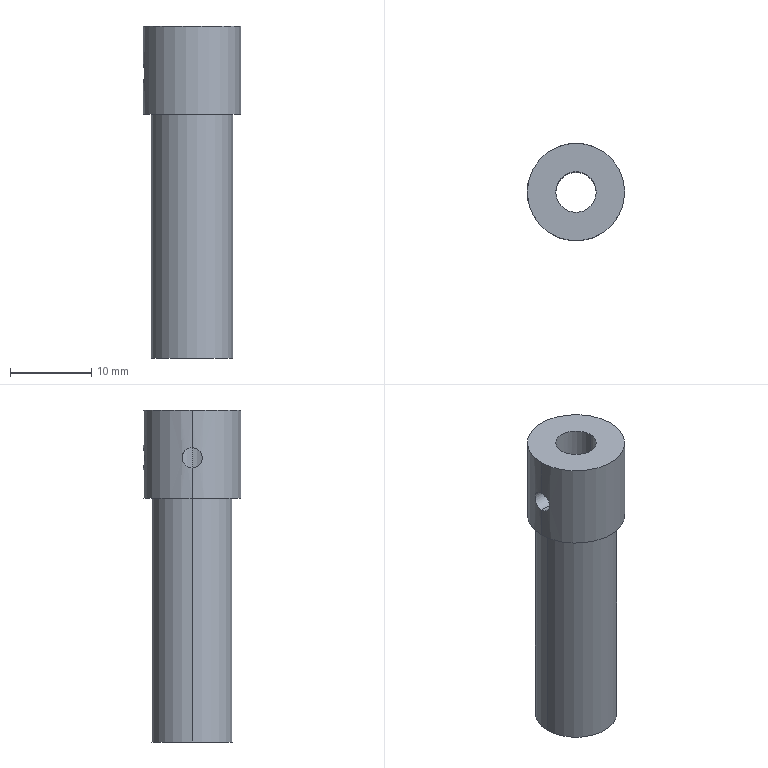Part | STEP file | 04-09 rotary shaft | 1 solid | 13 faces | box 12 x 12 x 40.9 mm | volume 2751 mm3 | cylinder 10 | plane 3 | commonest cylinder face diameters 2.5 x4 5 x2 10 x2 12 x2
STEP:
#1=CARTESIAN_POINT('',(-6.,0.,6.25));
#2=VERTEX_POINT('',#1);
#3=CARTESIAN_POINT('',(-6.,0.,3.75));
#4=VERTEX_POINT('',#3);
#5=CARTESIAN_POINT('',(-6.,0.,6.25));
#6=CARTESIAN_POINT('',(-6.,-0.1657,6.25));
#7=CARTESIAN_POINT('',(-5.993,-0.3282,6.217));
#8=CARTESIAN_POINT('',(-5.969,-0.6308,6.092));
#9=CARTESIAN_POINT('',(-5.952,-0.7692,5.999));
#10=CARTESIAN_POINT('',(-5.917,-0.9991,5.769));
#11=CARTESIAN_POINT('',(-5.9,-1.092,5.63));
#12=CARTESIAN_POINT('',(-5.876,-1.217,5.329));
#13=CARTESIAN_POINT('',(-5.868,-1.25,5.164));
#14=CARTESIAN_POINT('',(-5.868,-1.25,4.919));
#15=CARTESIAN_POINT('',(-5.87,-1.242,4.836));
#16=CARTESIAN_POINT('',(-5.877,-1.21,4.675));
#17=CARTESIAN_POINT('',(-5.882,-1.186,4.597));
#18=CARTESIAN_POINT('',(-5.9,-1.092,4.37));
#19=CARTESIAN_POINT('',(-5.917,-0.9999,4.232));
#20=CARTESIAN_POINT('',(-5.952,-0.7677,4.));
#21=CARTESIAN_POINT('',(-5.969,-0.63,3.908));
#22=CARTESIAN_POINT('',(-5.993,-0.3278,3.783));
#23=CARTESIAN_POINT('',(-6.,-0.1634,3.75));
#24=CARTESIAN_POINT('',(-6.,0.,3.75));
#25=B_SPLINE_CURVE_WITH_KNOTS('',3,(#5,#6,#7,#8,#9,#10,#11,#12,#13,#14,#15,#16,#17,#18,#19,#20,#21,#22,#23,#24),.UNSPECIFIED.,.F.,.F.,(4,2,2,2,2,2,2,2,2,4),(0.,0.0004899,0.0009797,0.00147,0.001959,0.002204,0.002449,0.002939,0.003429,0.003919),.UNSPECIFIED.);
#26=EDGE_CURVE('',#2,#4,#25,.T.);
#27=ORIENTED_EDGE('',*,*,#26,.F.);
#28=CARTESIAN_POINT('',(-2.5,0.,6.25));
#29=VERTEX_POINT('',#28);
#30=CARTESIAN_POINT('',(0.,0.,6.25));
#31=DIRECTION('',(1.,0.,0.));
#32=VECTOR('',#31,1000.);
#33=LINE('',#30,#32);
#34=EDGE_CURVE('',#2,#29,#33,.T.);
#35=ORIENTED_EDGE('',*,*,#34,.T.);
#36=CARTESIAN_POINT('',(-2.5,0.,3.75));
#37=VERTEX_POINT('',#36);
#38=CARTESIAN_POINT('',(-2.5,0.,3.75));
#39=CARTESIAN_POINT('',(-2.5,-0.08412,3.75));
#40=CARTESIAN_POINT('',(-2.496,-0.1666,3.758));
#41=CARTESIAN_POINT('',(-2.48,-0.3284,3.791));
#42=CARTESIAN_POINT('',(-2.468,-0.4085,3.816));
#43=CARTESIAN_POINT('',(-2.423,-0.635,3.911));
#44=CARTESIAN_POINT('',(-2.381,-0.7717,4.004));
#45=CARTESIAN_POINT('',(-2.295,-0.9981,4.231));
#46=CARTESIAN_POINT('',(-2.251,-1.09,4.367));
#47=CARTESIAN_POINT('',(-2.202,-1.184,4.592));
#48=CARTESIAN_POINT('',(-2.188,-1.209,4.672));
#49=CARTESIAN_POINT('',(-2.17,-1.242,4.834));
#50=CARTESIAN_POINT('',(-2.165,-1.25,4.916));
#51=CARTESIAN_POINT('',(-2.165,-1.25,5.165));
#52=CARTESIAN_POINT('',(-2.185,-1.216,5.332));
#53=CARTESIAN_POINT('',(-2.251,-1.089,5.634));
#54=CARTESIAN_POINT('',(-2.296,-0.9974,5.77));
#55=CARTESIAN_POINT('',(-2.381,-0.7706,5.997));
#56=CARTESIAN_POINT('',(-2.423,-0.6332,6.09));
#57=CARTESIAN_POINT('',(-2.482,-0.3331,6.216));
#58=CARTESIAN_POINT('',(-2.5,-0.166,6.25));
#59=CARTESIAN_POINT('',(-2.5,0.,6.25));
#60=B_SPLINE_CURVE_WITH_KNOTS('',3,(#38,#39,#40,#41,#42,#43,#44,#45,#46,#47,#48,#49,#50,#51,#52,#53,#54,#55,#56,#57,#58,#59),.UNSPECIFIED.,.F.,.F.,(4,2,2,2,2,2,2,2,2,2,4),(0.,0.0002485,0.000497,0.0009941,0.001491,0.00174,0.001988,0.002485,0.002982,0.003479,0.003976),.UNSPECIFIED.);
#61=EDGE_CURVE('',#37,#29,#60,.T.);
#62=ORIENTED_EDGE('',*,*,#61,.F.);
#63=CARTESIAN_POINT('',(0.,0.,3.75));
#64=DIRECTION('',(1.,0.,0.));
#65=VECTOR('',#64,1000.);
#66=LINE('',#63,#65);
#67=EDGE_CURVE('',#4,#37,#66,.T.);
#68=ORIENTED_EDGE('',*,*,#67,.F.);
#69=EDGE_LOOP('',(#27,#35,#62,#68));
#70=FACE_OUTER_BOUND('',#69,.T.);
#71=CARTESIAN_POINT('',(0.,0.,5.));
#72=DIRECTION('',(1.,0.,0.));
#73=DIRECTION('',(0.,0.,-1.));
#74=AXIS2_PLACEMENT_3D('',#71,#72,#73);
#75=CYLINDRICAL_SURFACE('',#74,1.25);
#76=ADVANCED_FACE('',(#70),#75,.F.);
#77=CARTESIAN_POINT('',(0.,6.,6.25));
#78=VERTEX_POINT('',#77);
#79=CARTESIAN_POINT('',(0.,6.,3.75));
#80=VERTEX_POINT('',#79);
#81=CARTESIAN_POINT('',(0.,6.,6.25));
#82=CARTESIAN_POINT('',(-0.1634,6.,6.25));
#83=CARTESIAN_POINT('',(-0.3283,5.993,6.217));
#84=CARTESIAN_POINT('',(-0.6292,5.969,6.092));
#85=CARTESIAN_POINT('',(-0.7681,5.952,6.));
#86=CARTESIAN_POINT('',(-0.9987,5.917,5.769));
#87=CARTESIAN_POINT('',(-1.091,5.9,5.632));
#88=CARTESIAN_POINT('',(-1.217,5.876,5.328));
#89=CARTESIAN_POINT('',(-1.25,5.868,5.166));
#90=CARTESIAN_POINT('',(-1.25,5.868,4.836));
#91=CARTESIAN_POINT('',(-1.217,5.876,4.672));
#92=CARTESIAN_POINT('',(-1.092,5.9,4.37));
#93=CARTESIAN_POINT('',(-0.9992,5.917,4.232));
#94=CARTESIAN_POINT('',(-0.7697,5.952,4.002));
#95=CARTESIAN_POINT('',(-0.6307,5.969,3.909));
#96=CARTESIAN_POINT('',(-0.33,5.993,3.783));
#97=CARTESIAN_POINT('',(-0.1656,6.,3.75));
#98=CARTESIAN_POINT('',(0.,6.,3.75));
#99=B_SPLINE_CURVE_WITH_KNOTS('',3,(#81,#82,#83,#84,#85,#86,#87,#88,#89,#90,#91,#92,#93,#94,#95,#96,#97,#98),.UNSPECIFIED.,.F.,.F.,(4,2,2,2,2,2,2,2,4),(0.003919,0.004409,0.004898,0.005388,0.005878,0.006367,0.006857,0.007347,0.007837),.UNSPECIFIED.);
#100=EDGE_CURVE('',#78,#80,#99,.T.);
#101=ORIENTED_EDGE('',*,*,#100,.F.);
#102=CARTESIAN_POINT('',(0.,2.5,6.25));
#103=VERTEX_POINT('',#102);
#104=CARTESIAN_POINT('',(0.,0.,6.25));
#105=DIRECTION('',(0.,-1.,0.));
#106=VECTOR('',#105,1000.);
#107=LINE('',#104,#106);
#108=EDGE_CURVE('',#78,#103,#107,.T.);
#109=ORIENTED_EDGE('',*,*,#108,.T.);
#110=CARTESIAN_POINT('',(0.,2.5,3.75));
#111=VERTEX_POINT('',#110);
#112=CARTESIAN_POINT('',(0.,2.5,3.75));
#113=CARTESIAN_POINT('',(-0.08412,2.5,3.75));
#114=CARTESIAN_POINT('',(-0.1666,2.496,3.758));
#115=CARTESIAN_POINT('',(-0.3284,2.48,3.791));
#116=CARTESIAN_POINT('',(-0.4085,2.468,3.816));
#117=CARTESIAN_POINT('',(-0.635,2.423,3.911));
#118=CARTESIAN_POINT('',(-0.7717,2.381,4.004));
#119=CARTESIAN_POINT('',(-0.9981,2.295,4.231));
#120=CARTESIAN_POINT('',(-1.09,2.251,4.367));
#121=CARTESIAN_POINT('',(-1.184,2.202,4.592));
#122=CARTESIAN_POINT('',(-1.209,2.188,4.672));
#123=CARTESIAN_POINT('',(-1.242,2.17,4.834));
#124=CARTESIAN_POINT('',(-1.25,2.165,4.916));
#125=CARTESIAN_POINT('',(-1.25,2.165,5.165));
#126=CARTESIAN_POINT('',(-1.216,2.185,5.332));
#127=CARTESIAN_POINT('',(-1.089,2.251,5.634));
#128=CARTESIAN_POINT('',(-0.9974,2.296,5.77));
#129=CARTESIAN_POINT('',(-0.7706,2.381,5.997));
#130=CARTESIAN_POINT('',(-0.6332,2.423,6.09));
#131=CARTESIAN_POINT('',(-0.3331,2.482,6.216));
#132=CARTESIAN_POINT('',(-0.166,2.5,6.25));
#133=CARTESIAN_POINT('',(0.,2.5,6.25));
#134=B_SPLINE_CURVE_WITH_KNOTS('',3,(#112,#113,#114,#115,#116,#117,#118,#119,#120,#121,#122,#123,#124,#125,#126,#127,#128,#129,#130,#131,#132,#133),.UNSPECIFIED.,.F.,.F.,(4,2,2,2,2,2,2,2,2,2,4),(0.,0.0002485,0.000497,0.0009941,0.001491,0.00174,0.001988,0.002485,0.002982,0.003479,0.003976),.UNSPECIFIED.);
#135=EDGE_CURVE('',#111,#103,#134,.T.);
#136=ORIENTED_EDGE('',*,*,#135,.F.);
#137=CARTESIAN_POINT('',(0.,0.,3.75));
#138=DIRECTION('',(0.,-1.,0.));
#139=VECTOR('',#138,1000.);
#140=LINE('',#137,#139);
#141=EDGE_CURVE('',#80,#111,#140,.T.);
#142=ORIENTED_EDGE('',*,*,#141,.F.);
#143=EDGE_LOOP('',(#101,#109,#136,#142));
#144=FACE_OUTER_BOUND('',#143,.T.);
#145=CARTESIAN_POINT('',(0.,0.,5.));
#146=DIRECTION('',(0.,-1.,0.));
#147=DIRECTION('',(0.,0.,-1.));
#148=AXIS2_PLACEMENT_3D('',#145,#146,#147);
#149=CYLINDRICAL_SURFACE('',#148,1.25);
#150=ADVANCED_FACE('',(#144),#149,.F.);
#151=CARTESIAN_POINT('',(2.5,0.,-30.));
#152=VERTEX_POINT('',#151);
#153=CARTESIAN_POINT('',(-2.5,0.,-30.));
#154=VERTEX_POINT('',#153);
#155=CARTESIAN_POINT('',(0.,0.,-30.));
#156=DIRECTION('',(0.,0.,-1.));
#157=DIRECTION('',(-1.,0.,0.));
#158=AXIS2_PLACEMENT_3D('',#155,#156,#157);
#159=CIRCLE('',#158,2.5);
#160=EDGE_CURVE('',#152,#154,#159,.T.);
#161=ORIENTED_EDGE('',*,*,#160,.T.);
#162=CARTESIAN_POINT('',(-2.5,0.,-33.1));
#163=DIRECTION('',(0.,0.,1.));
#164=VECTOR('',#163,1000.);
#165=LINE('',#162,#164);
#166=EDGE_CURVE('',#154,#37,#165,.T.);
#167=ORIENTED_EDGE('',*,*,#166,.T.);
#168=ORIENTED_EDGE('',*,*,#61,.T.);
#169=CARTESIAN_POINT('',(-2.5,0.,10.9));
#170=VERTEX_POINT('',#169);
#171=CARTESIAN_POINT('',(-2.5,0.,-33.1));
#172=DIRECTION('',(0.,0.,1.));
#173=VECTOR('',#172,1000.);
#174=LINE('',#171,#173);
#175=EDGE_CURVE('',#29,#170,#174,.T.);
#176=ORIENTED_EDGE('',*,*,#175,.T.);
#177=CARTESIAN_POINT('',(2.5,0.,10.9));
#178=VERTEX_POINT('',#177);
#179=CARTESIAN_POINT('',(0.,0.,10.9));
#180=DIRECTION('',(0.,0.,1.));
#181=DIRECTION('',(1.,0.,0.));
#182=AXIS2_PLACEMENT_3D('',#179,#180,#181);
#183=CIRCLE('',#182,2.5);
#184=EDGE_CURVE('',#170,#178,#183,.T.);
#185=ORIENTED_EDGE('',*,*,#184,.T.);
#186=CARTESIAN_POINT('',(2.5,0.,-33.1));
#187=DIRECTION('',(0.,0.,1.));
#188=VECTOR('',#187,1000.);
#189=LINE('',#186,#188);
#190=EDGE_CURVE('',#152,#178,#189,.T.);
#191=ORIENTED_EDGE('',*,*,#190,.F.);
#192=EDGE_LOOP('',(#161,#167,#168,#176,#185,#191));
#193=FACE_OUTER_BOUND('',#192,.T.);
#194=CARTESIAN_POINT('',(0.,0.,-33.1));
#195=DIRECTION('',(0.,0.,1.));
#196=DIRECTION('',(1.,0.,0.));
#197=AXIS2_PLACEMENT_3D('',#194,#195,#196);
#198=CYLINDRICAL_SURFACE('',#197,2.5);
#199=ADVANCED_FACE('',(#193),#198,.F.);
#200=CARTESIAN_POINT('',(-5.,0.,-30.));
#201=VERTEX_POINT('',#200);
#202=CARTESIAN_POINT('',(5.,0.,-30.));
#203=VERTEX_POINT('',#202);
#204=CARTESIAN_POINT('',(0.,0.,-30.));
#205=DIRECTION('',(0.,0.,-1.));
#206=DIRECTION('',(-1.,0.,0.));
#207=AXIS2_PLACEMENT_3D('',#204,#205,#206);
#208=CIRCLE('',#207,5.);
#209=EDGE_CURVE('',#201,#203,#208,.T.);
#210=ORIENTED_EDGE('',*,*,#209,.F.);
#211=CARTESIAN_POINT('',(-5.,0.,0.));
#212=VERTEX_POINT('',#211);
#213=CARTESIAN_POINT('',(-5.,0.,-30.));
#214=DIRECTION('',(0.,0.,1.));
#215=VECTOR('',#214,1000.);
#216=LINE('',#213,#215);
#217=EDGE_CURVE('',#201,#212,#216,.T.);
#218=ORIENTED_EDGE('',*,*,#217,.T.);
#219=CARTESIAN_POINT('',(5.,0.,0.));
#220=VERTEX_POINT('',#219);
#221=CARTESIAN_POINT('',(0.,0.,0.));
#222=DIRECTION('',(0.,0.,-1.));
#223=DIRECTION('',(1.,0.,0.));
#224=AXIS2_PLACEMENT_3D('',#221,#222,#223);
#225=CIRCLE('',#224,5.);
#226=EDGE_CURVE('',#212,#220,#225,.T.);
#227=ORIENTED_EDGE('',*,*,#226,.T.);
#228=CARTESIAN_POINT('',(5.,0.,-30.));
#229=DIRECTION('',(0.,0.,1.));
#230=VECTOR('',#229,1000.);
#231=LINE('',#228,#230);
#232=EDGE_CURVE('',#203,#220,#231,.T.);
#233=ORIENTED_EDGE('',*,*,#232,.F.);
#234=EDGE_LOOP('',(#210,#218,#227,#233));
#235=FACE_OUTER_BOUND('',#234,.T.);
#236=CARTESIAN_POINT('',(0.,0.,-30.));
#237=DIRECTION('',(0.,0.,1.));
#238=DIRECTION('',(1.,0.,0.));
#239=AXIS2_PLACEMENT_3D('',#236,#237,#238);
#240=CYLINDRICAL_SURFACE('',#239,5.);
#241=ADVANCED_FACE('',(#235),#240,.T.);
#242=CARTESIAN_POINT('',(0.,6.,3.75));
#243=CARTESIAN_POINT('',(0.1657,6.,3.75));
#244=CARTESIAN_POINT('',(0.3282,5.993,3.783));
#245=CARTESIAN_POINT('',(0.6308,5.969,3.908));
#246=CARTESIAN_POINT('',(0.7692,5.952,4.001));
#247=CARTESIAN_POINT('',(0.9991,5.917,4.231));
#248=CARTESIAN_POINT('',(1.092,5.9,4.37));
#249=CARTESIAN_POINT('',(1.217,5.876,4.671));
#250=CARTESIAN_POINT('',(1.25,5.868,4.836));
#251=CARTESIAN_POINT('',(1.25,5.868,5.081));
#252=CARTESIAN_POINT('',(1.242,5.87,5.164));
#253=CARTESIAN_POINT('',(1.21,5.877,5.325));
#254=CARTESIAN_POINT('',(1.186,5.882,5.403));
#255=CARTESIAN_POINT('',(1.092,5.9,5.63));
#256=CARTESIAN_POINT('',(0.9999,5.917,5.768));
#257=CARTESIAN_POINT('',(0.7677,5.952,6.));
#258=CARTESIAN_POINT('',(0.63,5.969,6.092));
#259=CARTESIAN_POINT('',(0.3278,5.993,6.217));
#260=CARTESIAN_POINT('',(0.1634,6.,6.25));
#261=CARTESIAN_POINT('',(0.,6.,6.25));
#262=B_SPLINE_CURVE_WITH_KNOTS('',3,(#242,#243,#244,#245,#246,#247,#248,#249,#250,#251,#252,#253,#254,#255,#256,#257,#258,#259,#260,#261),.UNSPECIFIED.,.F.,.F.,(4,2,2,2,2,2,2,2,2,4),(0.,0.0004899,0.0009797,0.00147,0.001959,0.002204,0.002449,0.002939,0.003429,0.003919),.UNSPECIFIED.);
#263=EDGE_CURVE('',#80,#78,#262,.T.);
#264=ORIENTED_EDGE('',*,*,#263,.T.);
#265=ORIENTED_EDGE('',*,*,#100,.T.);
#266=EDGE_LOOP('',(#264,#265));
#267=FACE_BOUND('',#266,.T.);
#268=CARTESIAN_POINT('',(6.,0.,10.9));
#269=VERTEX_POINT('',#268);
#270=CARTESIAN_POINT('',(-6.,0.,10.9));
#271=VERTEX_POINT('',#270);
#272=CARTESIAN_POINT('',(0.,0.,10.9));
#273=DIRECTION('',(0.,0.,1.));
#274=DIRECTION('',(1.,0.,0.));
#275=AXIS2_PLACEMENT_3D('',#272,#273,#274);
#276=CIRCLE('',#275,6.);
#277=EDGE_CURVE('',#269,#271,#276,.T.);
#278=ORIENTED_EDGE('',*,*,#277,.F.);
#279=CARTESIAN_POINT('',(6.,0.,0.));
#280=VERTEX_POINT('',#279);
#281=CARTESIAN_POINT('',(6.,0.,10.9));
#282=DIRECTION('',(0.,0.,-1.));
#283=VECTOR('',#282,1000.);
#284=LINE('',#281,#283);
#285=EDGE_CURVE('',#269,#280,#284,.T.);
#286=ORIENTED_EDGE('',*,*,#285,.T.);
#287=CARTESIAN_POINT('',(-6.,0.,0.));
#288=VERTEX_POINT('',#287);
#289=CARTESIAN_POINT('',(0.,0.,0.));
#290=DIRECTION('',(0.,0.,1.));
#291=DIRECTION('',(1.,0.,0.));
#292=AXIS2_PLACEMENT_3D('',#289,#290,#291);
#293=CIRCLE('',#292,6.);
#294=EDGE_CURVE('',#280,#288,#293,.T.);
#295=ORIENTED_EDGE('',*,*,#294,.T.);
#296=CARTESIAN_POINT('',(-6.,0.,10.9));
#297=DIRECTION('',(0.,0.,-1.));
#298=VECTOR('',#297,1000.);
#299=LINE('',#296,#298);
#300=EDGE_CURVE('',#4,#288,#299,.T.);
#301=ORIENTED_EDGE('',*,*,#300,.F.);
#302=CARTESIAN_POINT('',(-6.,0.,3.75));
#303=CARTESIAN_POINT('',(-6.,0.1634,3.75));
#304=CARTESIAN_POINT('',(-5.993,0.3283,3.783));
#305=CARTESIAN_POINT('',(-5.969,0.6292,3.908));
#306=CARTESIAN_POINT('',(-5.952,0.7681,4.));
#307=CARTESIAN_POINT('',(-5.917,0.9987,4.231));
#308=CARTESIAN_POINT('',(-5.9,1.091,4.368));
#309=CARTESIAN_POINT('',(-5.876,1.217,4.672));
#310=CARTESIAN_POINT('',(-5.868,1.25,4.834));
#311=CARTESIAN_POINT('',(-5.868,1.25,5.164));
#312=CARTESIAN_POINT('',(-5.876,1.217,5.328));
#313=CARTESIAN_POINT('',(-5.9,1.092,5.63));
#314=CARTESIAN_POINT('',(-5.917,0.9992,5.768));
#315=CARTESIAN_POINT('',(-5.952,0.7697,5.998));
#316=CARTESIAN_POINT('',(-5.969,0.6307,6.091));
#317=CARTESIAN_POINT('',(-5.993,0.33,6.217));
#318=CARTESIAN_POINT('',(-6.,0.1656,6.25));
#319=CARTESIAN_POINT('',(-6.,0.,6.25));
#320=B_SPLINE_CURVE_WITH_KNOTS('',3,(#302,#303,#304,#305,#306,#307,#308,#309,#310,#311,#312,#313,#314,#315,#316,#317,#318,#319),.UNSPECIFIED.,.F.,.F.,(4,2,2,2,2,2,2,2,4),(0.003919,0.004409,0.004898,0.005388,0.005878,0.006367,0.006857,0.007347,0.007837),.UNSPECIFIED.);
#321=EDGE_CURVE('',#4,#2,#320,.T.);
#322=ORIENTED_EDGE('',*,*,#321,.T.);
#323=CARTESIAN_POINT('',(-6.,0.,10.9));
#324=DIRECTION('',(0.,0.,-1.));
#325=VECTOR('',#324,1000.);
#326=LINE('',#323,#325);
#327=EDGE_CURVE('',#271,#2,#326,.T.);
#328=ORIENTED_EDGE('',*,*,#327,.F.);
#329=EDGE_LOOP('',(#278,#286,#295,#301,#322,#328));
#330=FACE_OUTER_BOUND('',#329,.T.);
#331=CARTESIAN_POINT('',(0.,0.,10.9));
#332=DIRECTION('',(0.,0.,-1.));
#333=DIRECTION('',(-1.,0.,0.));
#334=AXIS2_PLACEMENT_3D('',#331,#332,#333);
#335=CYLINDRICAL_SURFACE('',#334,6.);
#336=ADVANCED_FACE('',(#267,#330),#335,.T.);
#337=CARTESIAN_POINT('',(0.,0.,0.));
#338=DIRECTION('',(0.,0.,1.));
#339=DIRECTION('',(1.,0.,0.));
#340=AXIS2_PLACEMENT_3D('',#337,#338,#339);
#341=CIRCLE('',#340,6.);
#342=EDGE_CURVE('',#288,#280,#341,.T.);
#343=ORIENTED_EDGE('',*,*,#342,.F.);
#344=ORIENTED_EDGE('',*,*,#294,.F.);
#345=EDGE_LOOP('',(#343,#344));
#346=FACE_OUTER_BOUND('',#345,.T.);
#347=CARTESIAN_POINT('',(0.,0.,0.));
#348=DIRECTION('',(0.,0.,-1.));
#349=DIRECTION('',(1.,0.,0.));
#350=AXIS2_PLACEMENT_3D('',#347,#348,#349);
#351=CIRCLE('',#350,5.);
#352=EDGE_CURVE('',#220,#212,#351,.T.);
#353=ORIENTED_EDGE('',*,*,#352,.F.);
#354=ORIENTED_EDGE('',*,*,#226,.F.);
#355=EDGE_LOOP('',(#353,#354));
#356=FACE_BOUND('',#355,.T.);
#357=CARTESIAN_POINT('',(0.,0.,0.));
#358=DIRECTION('',(0.,0.,1.));
#359=DIRECTION('',(1.,0.,0.));
#360=AXIS2_PLACEMENT_3D('',#357,#358,#359);
#361=PLANE('',#360);
#362=ADVANCED_FACE('',(#346,#356),#361,.F.);
#363=ORIENTED_EDGE('',*,*,#285,.F.);
#364=CARTESIAN_POINT('',(0.,0.,10.9));
#365=DIRECTION('',(0.,0.,1.));
#366=DIRECTION('',(1.,0.,0.));
#367=AXIS2_PLACEMENT_3D('',#364,#365,#366);
#368=CIRCLE('',#367,6.);
#369=EDGE_CURVE('',#271,#269,#368,.T.);
#370=ORIENTED_EDGE('',*,*,#369,.F.);
#371=ORIENTED_EDGE('',*,*,#327,.T.);
#372=ORIENTED_EDGE('',*,*,#26,.T.);
#373=ORIENTED_EDGE('',*,*,#300,.T.);
#374=ORIENTED_EDGE('',*,*,#342,.T.);
#375=EDGE_LOOP('',(#363,#370,#371,#372,#373,#374));
#376=FACE_OUTER_BOUND('',#375,.T.);
#377=CARTESIAN_POINT('',(0.,0.,10.9));
#378=DIRECTION('',(0.,0.,-1.));
#379=DIRECTION('',(-1.,0.,0.));
#380=AXIS2_PLACEMENT_3D('',#377,#378,#379);
#381=CYLINDRICAL_SURFACE('',#380,6.);
#382=ADVANCED_FACE('',(#376),#381,.T.);
#383=CARTESIAN_POINT('',(0.,0.,10.9));
#384=DIRECTION('',(0.,0.,1.));
#385=DIRECTION('',(1.,0.,0.));
#386=AXIS2_PLACEMENT_3D('',#383,#384,#385);
#387=CIRCLE('',#386,2.5);
#388=EDGE_CURVE('',#178,#170,#387,.T.);
#389=ORIENTED_EDGE('',*,*,#388,.F.);
#390=ORIENTED_EDGE('',*,*,#184,.F.);
#391=EDGE_LOOP('',(#389,#390));
#392=FACE_BOUND('',#391,.T.);
#393=ORIENTED_EDGE('',*,*,#369,.T.);
#394=ORIENTED_EDGE('',*,*,#277,.T.);
#395=EDGE_LOOP('',(#393,#394));
#396=FACE_OUTER_BOUND('',#395,.T.);
#397=CARTESIAN_POINT('',(0.,0.,10.9));
#398=DIRECTION('',(0.,0.,1.));
#399=DIRECTION('',(1.,0.,0.));
#400=AXIS2_PLACEMENT_3D('',#397,#398,#399);
#401=PLANE('',#400);
#402=ADVANCED_FACE('',(#392,#396),#401,.T.);
#403=ORIENTED_EDGE('',*,*,#217,.F.);
#404=CARTESIAN_POINT('',(0.,0.,-30.));
#405=DIRECTION('',(0.,0.,-1.));
#406=DIRECTION('',(-1.,0.,0.));
#407=AXIS2_PLACEMENT_3D('',#404,#405,#406);
#408=CIRCLE('',#407,5.);
#409=EDGE_CURVE('',#203,#201,#408,.T.);
#410=ORIENTED_EDGE('',*,*,#409,.F.);
#411=ORIENTED_EDGE('',*,*,#232,.T.);
#412=ORIENTED_EDGE('',*,*,#352,.T.);
#413=EDGE_LOOP('',(#403,#410,#411,#412));
#414=FACE_OUTER_BOUND('',#413,.T.);
#415=CARTESIAN_POINT('',(0.,0.,-30.));
#416=DIRECTION('',(0.,0.,1.));
#417=DIRECTION('',(1.,0.,0.));
#418=AXIS2_PLACEMENT_3D('',#415,#416,#417);
#419=CYLINDRICAL_SURFACE('',#418,5.);
#420=ADVANCED_FACE('',(#414),#419,.T.);
#421=ORIENTED_EDGE('',*,*,#160,.F.);
#422=CARTESIAN_POINT('',(0.,0.,-30.));
#423=DIRECTION('',(0.,0.,-1.));
#424=DIRECTION('',(-1.,0.,0.));
#425=AXIS2_PLACEMENT_3D('',#422,#423,#424);
#426=CIRCLE('',#425,2.5);
#427=EDGE_CURVE('',#154,#152,#426,.T.);
#428=ORIENTED_EDGE('',*,*,#427,.F.);
#429=EDGE_LOOP('',(#421,#428));
#430=FACE_BOUND('',#429,.T.);
#431=ORIENTED_EDGE('',*,*,#409,.T.);
#432=ORIENTED_EDGE('',*,*,#209,.T.);
#433=EDGE_LOOP('',(#431,#432));
#434=FACE_OUTER_BOUND('',#433,.T.);
#435=CARTESIAN_POINT('',(0.,0.,-30.));
#436=DIRECTION('',(0.,0.,-1.));
#437=DIRECTION('',(-1.,0.,0.));
#438=AXIS2_PLACEMENT_3D('',#435,#436,#437);
#439=PLANE('',#438);
#440=ADVANCED_FACE('',(#430,#434),#439,.T.);
#441=ORIENTED_EDGE('',*,*,#166,.F.);
#442=ORIENTED_EDGE('',*,*,#427,.T.);
#443=ORIENTED_EDGE('',*,*,#190,.T.);
#444=ORIENTED_EDGE('',*,*,#388,.T.);
#445=ORIENTED_EDGE('',*,*,#175,.F.);
#446=CARTESIAN_POINT('',(-2.5,0.,6.25));
#447=CARTESIAN_POINT('',(-2.5,0.08285,6.25));
#448=CARTESIAN_POINT('',(-2.496,0.1672,6.242));
#449=CARTESIAN_POINT('',(-2.48,0.3292,6.209));
#450=CARTESIAN_POINT('',(-2.468,0.4077,6.185));
#451=CARTESIAN_POINT('',(-2.423,0.6361,6.089));
#452=CARTESIAN_POINT('',(-2.381,0.7717,5.996));
#453=CARTESIAN_POINT('',(-2.295,0.9986,5.769));
#454=CARTESIAN_POINT('',(-2.251,1.09,5.632));
#455=CARTESIAN_POINT('',(-2.186,1.216,5.333));
#456=CARTESIAN_POINT('',(-2.165,1.25,5.167));
#457=CARTESIAN_POINT('',(-2.165,1.25,4.836));
#458=CARTESIAN_POINT('',(-2.185,1.217,4.669));
#459=CARTESIAN_POINT('',(-2.251,1.09,4.367));
#460=CARTESIAN_POINT('',(-2.295,0.9987,4.231));
#461=CARTESIAN_POINT('',(-2.36,0.8277,4.06));
#462=CARTESIAN_POINT('',(-2.381,0.7659,4.009));
#463=CARTESIAN_POINT('',(-2.42,0.6321,3.919));
#464=CARTESIAN_POINT('',(-2.438,0.5593,3.879));
#465=CARTESIAN_POINT('',(-2.482,0.3335,3.784));
#466=CARTESIAN_POINT('',(-2.5,0.168,3.75));
#467=CARTESIAN_POINT('',(-2.5,0.,3.75));
#468=B_SPLINE_CURVE_WITH_KNOTS('',3,(#446,#447,#448,#449,#450,#451,#452,#453,#454,#455,#456,#457,#458,#459,#460,#461,#462,#463,#464,#465,#466,#467),.UNSPECIFIED.,.F.,.F.,(4,2,2,2,2,2,2,2,2,2,4),(0.003976,0.004224,0.004472,0.004969,0.005465,0.005961,0.006457,0.006953,0.007201,0.007449,0.007946),.UNSPECIFIED.);
#469=EDGE_CURVE('',#29,#37,#468,.T.);
#470=ORIENTED_EDGE('',*,*,#469,.T.);
#471=EDGE_LOOP('',(#441,#442,#443,#444,#445,#470));
#472=FACE_OUTER_BOUND('',#471,.T.);
#473=ORIENTED_EDGE('',*,*,#135,.T.);
#474=CARTESIAN_POINT('',(0.,2.5,6.25));
#475=CARTESIAN_POINT('',(0.08285,2.5,6.25));
#476=CARTESIAN_POINT('',(0.1672,2.496,6.242));
#477=CARTESIAN_POINT('',(0.3292,2.48,6.209));
#478=CARTESIAN_POINT('',(0.4077,2.468,6.185));
#479=CARTESIAN_POINT('',(0.6361,2.423,6.089));
#480=CARTESIAN_POINT('',(0.7717,2.381,5.996));
#481=CARTESIAN_POINT('',(0.9986,2.295,5.769));
#482=CARTESIAN_POINT('',(1.09,2.251,5.632));
#483=CARTESIAN_POINT('',(1.216,2.186,5.333));
#484=CARTESIAN_POINT('',(1.25,2.165,5.167));
#485=CARTESIAN_POINT('',(1.25,2.165,4.836));
#486=CARTESIAN_POINT('',(1.217,2.185,4.669));
#487=CARTESIAN_POINT('',(1.09,2.251,4.367));
#488=CARTESIAN_POINT('',(0.9987,2.295,4.231));
#489=CARTESIAN_POINT('',(0.8277,2.36,4.06));
#490=CARTESIAN_POINT('',(0.7659,2.381,4.009));
#491=CARTESIAN_POINT('',(0.6321,2.42,3.919));
#492=CARTESIAN_POINT('',(0.5593,2.438,3.879));
#493=CARTESIAN_POINT('',(0.3335,2.482,3.784));
#494=CARTESIAN_POINT('',(0.168,2.5,3.75));
#495=CARTESIAN_POINT('',(0.,2.5,3.75));
#496=B_SPLINE_CURVE_WITH_KNOTS('',3,(#474,#475,#476,#477,#478,#479,#480,#481,#482,#483,#484,#485,#486,#487,#488,#489,#490,#491,#492,#493,#494,#495),.UNSPECIFIED.,.F.,.F.,(4,2,2,2,2,2,2,2,2,2,4),(0.003976,0.004224,0.004472,0.004969,0.005465,0.005961,0.006457,0.006953,0.007201,0.007449,0.007946),.UNSPECIFIED.);
#497=EDGE_CURVE('',#103,#111,#496,.T.);
#498=ORIENTED_EDGE('',*,*,#497,.T.);
#499=EDGE_LOOP('',(#473,#498));
#500=FACE_BOUND('',#499,.T.);
#501=CARTESIAN_POINT('',(0.,0.,-33.1));
#502=DIRECTION('',(0.,0.,1.));
#503=DIRECTION('',(1.,0.,0.));
#504=AXIS2_PLACEMENT_3D('',#501,#502,#503);
#505=CYLINDRICAL_SURFACE('',#504,2.5);
#506=ADVANCED_FACE('',(#472,#500),#505,.F.);
#507=ORIENTED_EDGE('',*,*,#108,.F.);
#508=ORIENTED_EDGE('',*,*,#263,.F.);
#509=ORIENTED_EDGE('',*,*,#141,.T.);
#510=ORIENTED_EDGE('',*,*,#497,.F.);
#511=EDGE_LOOP('',(#507,#508,#509,#510));
#512=FACE_OUTER_BOUND('',#511,.T.);
#513=CARTESIAN_POINT('',(0.,0.,5.));
#514=DIRECTION('',(0.,-1.,0.));
#515=DIRECTION('',(0.,0.,-1.));
#516=AXIS2_PLACEMENT_3D('',#513,#514,#515);
#517=CYLINDRICAL_SURFACE('',#516,1.25);
#518=ADVANCED_FACE('',(#512),#517,.F.);
#519=ORIENTED_EDGE('',*,*,#34,.F.);
#520=ORIENTED_EDGE('',*,*,#321,.F.);
#521=ORIENTED_EDGE('',*,*,#67,.T.);
#522=ORIENTED_EDGE('',*,*,#469,.F.);
#523=EDGE_LOOP('',(#519,#520,#521,#522));
#524=FACE_OUTER_BOUND('',#523,.T.);
#525=CARTESIAN_POINT('',(0.,0.,5.));
#526=DIRECTION('',(1.,0.,0.));
#527=DIRECTION('',(0.,0.,-1.));
#528=AXIS2_PLACEMENT_3D('',#525,#526,#527);
#529=CYLINDRICAL_SURFACE('',#528,1.25);
#530=ADVANCED_FACE('',(#524),#529,.F.);
#531=CLOSED_SHELL('',(#76,#150,#199,#241,#336,#362,#382,#402,#420,#440,#506,#518,#530));
#532=MANIFOLD_SOLID_BREP('',#531);
#533=CARTESIAN_POINT('',(0.,0.,0.));
#534=DIRECTION('',(0.,0.,1.));
#535=DIRECTION('',(1.,0.,0.));
#536=AXIS2_PLACEMENT_3D('',#533,#534,#535);
#537=(LENGTH_UNIT()NAMED_UNIT(*)SI_UNIT(.MILLI.,.METRE.));
#538=UNCERTAINTY_MEASURE_WITH_UNIT(LENGTH_MEASURE(0.00001),#537,'','');
#539=(NAMED_UNIT(*)PLANE_ANGLE_UNIT()SI_UNIT($,.RADIAN.));
#540=(NAMED_UNIT(*)SI_UNIT($,.STERADIAN.)SOLID_ANGLE_UNIT());
#541=(GEOMETRIC_REPRESENTATION_CONTEXT(3)GLOBAL_UNCERTAINTY_ASSIGNED_CONTEXT((#538))GLOBAL_UNIT_ASSIGNED_CONTEXT((#537,#539,#540))REPRESENTATION_CONTEXT('',''));
#542=ADVANCED_BREP_SHAPE_REPRESENTATION('',(#532,#536),#541);